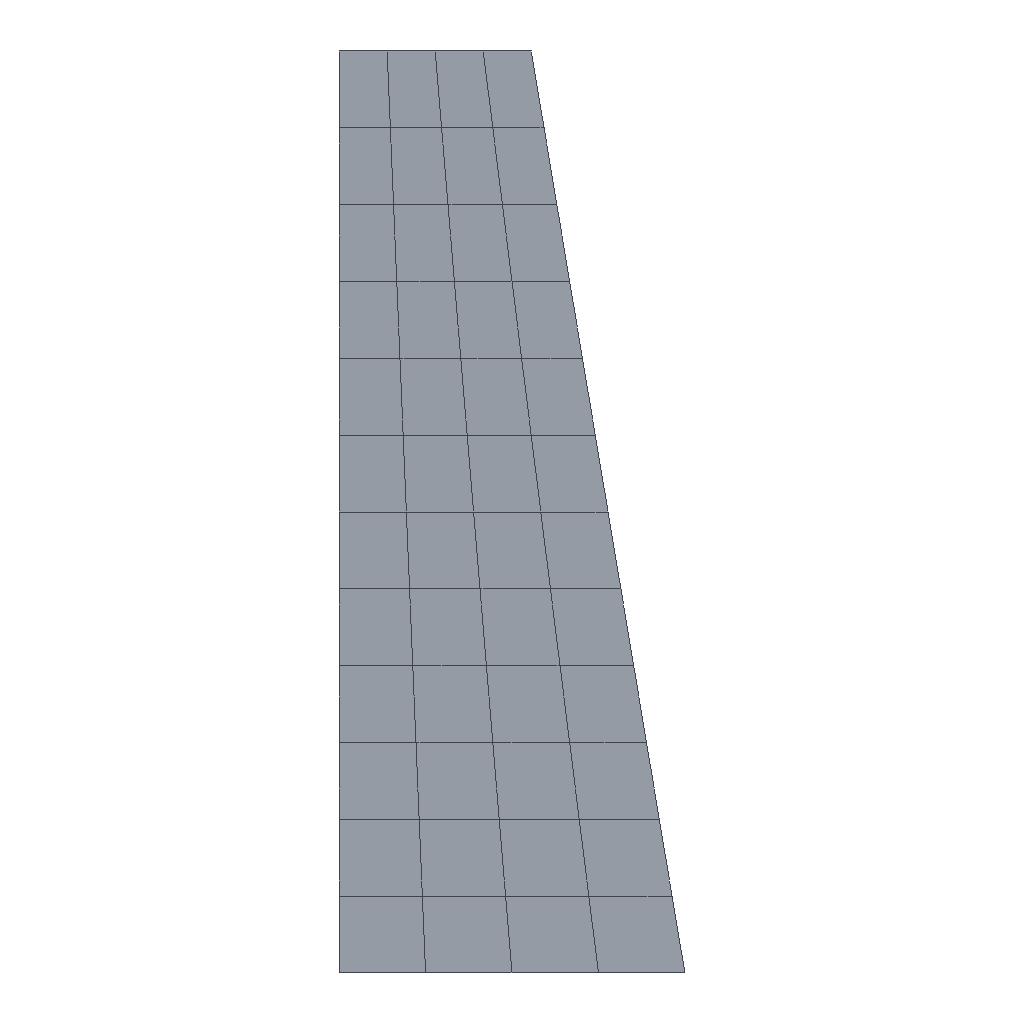Simulation study | abaqus
Set-up summary:
category,name,step,type,value,unit,region
solver,abaqus
solver,version,,,Abaqus/Standard 3DEXPERIENCE R2019x
units,not stated in the deck,,not stated
analysis,deck,,static,static
load_step,Step-1,Step-1,static
load_step,requested,,,1
mesh,nodes,,,77
mesh,elements,,,58
element_type,CPS4,,plane,48
element_type,R2D2,,rigid,10
load,load commands in deck,,count,1
bc,support commands in deck,,count,3
material,MATERIAL-1,,in results
check,setup vs results,,match,"per instance, exact: element labels, types and connectivity; labels of the nodes the elements use; coordinates of those nodes at SINGLE_PRECISION in 2 of 2 instance(s)"
Abaqus input file, long lists of numbers shortened:
*Heading
** Job name: Job-1 Model name: Model-1
** Generated by: Abaqus/CAE 2019
*Preprint, echo=NO, model=NO, history=NO, contact=NO
**
** PARTS
**
*Part, name=Part-1
*Node
      1,         13.5,           0.
      2,   14.8,           0.
** (9 more lines like these left out)
*Element, type=R2D2
 1,  1,  2
 2,  2,  3
** (8 more lines like these left out)
*Node
     12,          20.,           0.,           0.
*Nset, nset=Part-1-RefPt_, internal
12,
*Elset, elset=Part-1, generate
  1,  10,   1
*End Part
**
*Part, name=Part-2
*Node
      1,          4.5,          12.
      2,        3.875,          12.
** (63 more lines like these left out)
*Element, type=CPS4
 1,  1,  2,  7,  6
 2,  2,  3,  8,  7
** (46 more lines like these left out)
*Nset, nset=_PickedSet12, internal, generate
  1,  65,   1
*Elset, elset=_PickedSet12, internal, generate
  1,  48,   1
** Section: Section-1
*Solid Section, elset=_PickedSet12, material=Material-1
,
*End Part
**
**
** ASSEMBLY
**
*Assembly, name=Assembly
**
*Instance, name=Part-1-1, part=Part-1
       -11.5,           0.,           0.
*End Instance
**
*Instance, name=Part-2-1, part=Part-2
*End Instance
**
*Nset, nset=_PickedSet10, internal, instance=Part-2-1, generate
 1,  5,  1
*Elset, elset=_PickedSet10, internal, instance=Part-2-1, generate
 1,  4,  1
*Nset, nset=_PickedSet12, internal, instance=Part-1-1
 12,
*Nset, nset=_PickedSet13, internal, instance=Part-2-1, generate
  5,  65,   5
*Elset, elset=_PickedSet13, internal, instance=Part-2-1, generate
  4,  48,   4
*Elset, elset=__PickedSurf7_S3, internal, instance=Part-2-1, generate
 45,  48,   1
*Surface, type=ELEMENT, name=_PickedSurf7, internal
__PickedSurf7_S3, S3
*Elset, elset=__PickedSurf8_SPOS, internal, instance=Part-1-1, generate
  1,  10,   1
*Surface, type=ELEMENT, name=_PickedSurf8, internal
__PickedSurf8_SPOS, SPOS
*Rigid Body, ref node=Part-1-1.Part-1-RefPt_, elset=Part-1-1.Part-1
*End Assembly
**
** MATERIALS
**
*Material, name=Material-1
*Hyperelastic, mooney-rivlin
 0.166, 0.144,    0.
**
** INTERACTION PROPERTIES
**
*Surface Interaction, name=IntProp-1
1.,
*Friction, slip tolerance=0.005
 0.8,
*Surface Behavior, pressure-overclosure=HARD
**
** BOUNDARY CONDITIONS
**
** Name: BC-3 Type: 对称/反对称/完全固定
*Boundary
_PickedSet12, ENCASTRE
**
** INTERACTIONS
**
** Interaction: Int-1
*Contact Pair, interaction=IntProp-1, type=SURFACE TO SURFACE
_PickedSurf7, _PickedSurf8
** ----------------------------------------------------------------
**
** STEP: Step-1
**
*Step, name=Step-1, nlgeom=YES
*Static
0.01, 1., 1e-05, 1.
**
** BOUNDARY CONDITIONS
**
** Name: BC-2 Type: 位移/转角
*Boundary
_PickedSet10, 2, 2, -3.
** Name: BC-4 Type: 对称/反对称/完全固定
*Boundary
_PickedSet13, XSYMM
**
** OUTPUT REQUESTS
**
*Restart, write, frequency=0
**
** FIELD OUTPUT: F-Output-1
**
*Output, field
*Node Output
CF, RF, U
*Element Output, directions=YES
LE, NE, PE, PEEQ, PEMAG, S
*Contact Output
CDISP, CSTRESS
**
** HISTORY OUTPUT: H-Output-1
**
*Output, history, variable=PRESELECT
*End Step
Results summary:
result,step,,completed,increments=11 time=1.0/1.0
result,analysis,,,static
result,last_loadstep,,,1
result,primary field,,,U
result,reaction total,,FX,-0.0,model units
result,reaction total,,FY,-0.0,model units
result,reaction total,,FZ,0.0,model units